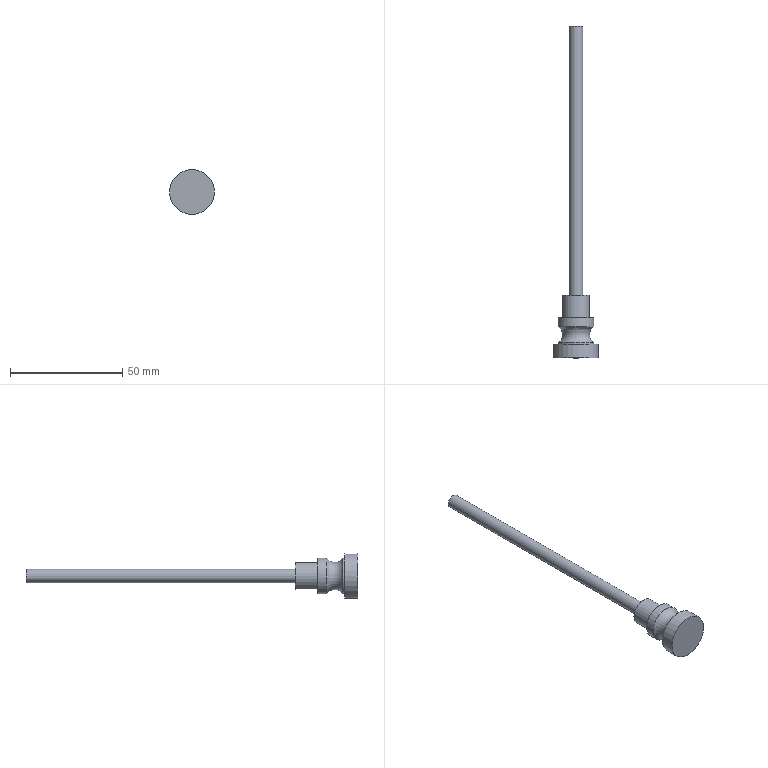Part | NX | features DATUM_CSYS 6, SKETCH 5, EXTRUDE 4, SWP104 1 | 1 solid | 11 faces | box 20 x 148 x 20 mm | volume 8375 mm3 | cylinder 5 | plane 5 | torus 1 | commonest cylinder face diameters 16 x2 6 x1 12 x1 20 x1
STEP:
#1=CARTESIAN_POINT('',(0.,0.721,8.));
#2=VERTEX_POINT('',#1);
#3=CARTESIAN_POINT('',(0.,0.721,0.));
#4=DIRECTION('',(0.,1.,0.));
#5=DIRECTION('',(0.,0.,1.));
#6=AXIS2_PLACEMENT_3D('',#3,#4,#5);
#7=CIRCLE('',#6,8.);
#8=EDGE_CURVE('',#2,#2,#7,.T.);
#9=ORIENTED_EDGE('',*,*,#8,.F.);
#10=EDGE_LOOP('',(#9));
#11=FACE_BOUND('',#10,.T.);
#12=CARTESIAN_POINT('',(8.,0.,0.));
#13=VERTEX_POINT('',#12);
#14=CARTESIAN_POINT('',(0.,0.,0.));
#15=DIRECTION('',(0.,1.,0.));
#16=DIRECTION('',(1.,0.,0.));
#17=AXIS2_PLACEMENT_3D('',#14,#15,#16);
#18=CIRCLE('',#17,8.);
#19=EDGE_CURVE('',#13,#13,#18,.T.);
#20=ORIENTED_EDGE('',*,*,#19,.T.);
#21=EDGE_LOOP('',(#20));
#22=FACE_BOUND('',#21,.T.);
#23=CARTESIAN_POINT('',(0.,12.,0.));
#24=DIRECTION('',(0.,-1.,0.));
#25=DIRECTION('',(0.,0.,-1.));
#26=AXIS2_PLACEMENT_3D('',#23,#24,#25);
#27=CYLINDRICAL_SURFACE('',#26,8.);
#28=ADVANCED_FACE('',(#11,#22),#27,.T.);
#29=CARTESIAN_POINT('',(10.,-6.,0.));
#30=VERTEX_POINT('',#29);
#31=CARTESIAN_POINT('',(0.,-6.,0.));
#32=DIRECTION('',(0.,-1.,0.));
#33=DIRECTION('',(1.,0.,0.));
#34=AXIS2_PLACEMENT_3D('',#31,#32,#33);
#35=CIRCLE('',#34,10.);
#36=EDGE_CURVE('',#30,#30,#35,.T.);
#37=ORIENTED_EDGE('',*,*,#36,.F.);
#38=EDGE_LOOP('',(#37));
#39=FACE_BOUND('',#38,.T.);
#40=CARTESIAN_POINT('',(10.,0.,0.));
#41=VERTEX_POINT('',#40);
#42=CARTESIAN_POINT('',(0.,0.,0.));
#43=DIRECTION('',(0.,-1.,0.));
#44=DIRECTION('',(1.,0.,0.));
#45=AXIS2_PLACEMENT_3D('',#42,#43,#44);
#46=CIRCLE('',#45,10.);
#47=EDGE_CURVE('',#41,#41,#46,.T.);
#48=ORIENTED_EDGE('',*,*,#47,.T.);
#49=EDGE_LOOP('',(#48));
#50=FACE_BOUND('',#49,.T.);
#51=CARTESIAN_POINT('',(0.,-6.,0.));
#52=DIRECTION('',(0.,1.,0.));
#53=DIRECTION('',(0.,0.,1.));
#54=AXIS2_PLACEMENT_3D('',#51,#52,#53);
#55=CYLINDRICAL_SURFACE('',#54,10.);
#56=ADVANCED_FACE('',(#39,#50),#55,.T.);
#57=ORIENTED_EDGE('',*,*,#36,.T.);
#58=EDGE_LOOP('',(#57));
#59=FACE_BOUND('',#58,.T.);
#60=CARTESIAN_POINT('',(0.,-6.,0.));
#61=DIRECTION('',(0.,-1.,0.));
#62=DIRECTION('',(0.,0.,-1.));
#63=AXIS2_PLACEMENT_3D('',#60,#61,#62);
#64=PLANE('',#63);
#65=ADVANCED_FACE('',(#59),#64,.T.);
#66=ORIENTED_EDGE('',*,*,#47,.F.);
#67=EDGE_LOOP('',(#66));
#68=FACE_BOUND('',#67,.T.);
#69=ORIENTED_EDGE('',*,*,#19,.F.);
#70=EDGE_LOOP('',(#69));
#71=FACE_BOUND('',#70,.T.);
#72=CARTESIAN_POINT('',(0.,0.,0.));
#73=DIRECTION('',(0.,-1.,0.));
#74=DIRECTION('',(0.,0.,-1.));
#75=AXIS2_PLACEMENT_3D('',#72,#73,#74);
#76=PLANE('',#75);
#77=ADVANCED_FACE('',(#68,#71),#76,.F.);
#78=CARTESIAN_POINT('',(0.,8.,-8.));
#79=VERTEX_POINT('',#78);
#80=CARTESIAN_POINT('',(0.,8.,0.));
#81=DIRECTION('',(0.,-1.,0.));
#82=DIRECTION('',(0.,0.,-1.));
#83=AXIS2_PLACEMENT_3D('',#80,#81,#82);
#84=CIRCLE('',#83,8.);
#85=EDGE_CURVE('',#79,#79,#84,.T.);
#86=ORIENTED_EDGE('',*,*,#85,.T.);
#87=EDGE_LOOP('',(#86));
#88=FACE_BOUND('',#87,.T.);
#89=ORIENTED_EDGE('',*,*,#8,.T.);
#90=EDGE_LOOP('',(#89));
#91=FACE_BOUND('',#90,.T.);
#92=CARTESIAN_POINT('',(0.,4.36,0.));
#93=DIRECTION('',(0.,-1.,0.));
#94=DIRECTION('',(0.,0.,-1.));
#95=AXIS2_PLACEMENT_3D('',#92,#93,#94);
#96=TOROIDAL_SURFACE('',#95,10.473,4.4);
#97=ADVANCED_FACE('',(#88,#91),#96,.F.);
#98=CARTESIAN_POINT('',(6.,12.,0.));
#99=VERTEX_POINT('',#98);
#100=CARTESIAN_POINT('',(0.,12.,0.));
#101=DIRECTION('',(0.,1.,0.));
#102=DIRECTION('',(1.,0.,0.));
#103=AXIS2_PLACEMENT_3D('',#100,#101,#102);
#104=CIRCLE('',#103,6.);
#105=EDGE_CURVE('',#99,#99,#104,.T.);
#106=ORIENTED_EDGE('',*,*,#105,.F.);
#107=EDGE_LOOP('',(#106));
#108=FACE_BOUND('',#107,.T.);
#109=CARTESIAN_POINT('',(8.,12.,0.));
#110=VERTEX_POINT('',#109);
#111=CARTESIAN_POINT('',(0.,12.,0.));
#112=DIRECTION('',(0.,1.,0.));
#113=DIRECTION('',(1.,0.,0.));
#114=AXIS2_PLACEMENT_3D('',#111,#112,#113);
#115=CIRCLE('',#114,8.);
#116=EDGE_CURVE('',#110,#110,#115,.T.);
#117=ORIENTED_EDGE('',*,*,#116,.T.);
#118=EDGE_LOOP('',(#117));
#119=FACE_BOUND('',#118,.T.);
#120=CARTESIAN_POINT('',(0.,12.,0.));
#121=DIRECTION('',(0.,1.,0.));
#122=DIRECTION('',(0.,0.,1.));
#123=AXIS2_PLACEMENT_3D('',#120,#121,#122);
#124=PLANE('',#123);
#125=ADVANCED_FACE('',(#108,#119),#124,.T.);
#126=ORIENTED_EDGE('',*,*,#85,.F.);
#127=EDGE_LOOP('',(#126));
#128=FACE_BOUND('',#127,.T.);
#129=ORIENTED_EDGE('',*,*,#116,.F.);
#130=EDGE_LOOP('',(#129));
#131=FACE_BOUND('',#130,.T.);
#132=CARTESIAN_POINT('',(0.,12.,0.));
#133=DIRECTION('',(0.,-1.,0.));
#134=DIRECTION('',(0.,0.,-1.));
#135=AXIS2_PLACEMENT_3D('',#132,#133,#134);
#136=CYLINDRICAL_SURFACE('',#135,8.);
#137=ADVANCED_FACE('',(#128,#131),#136,.T.);
#138=CARTESIAN_POINT('',(6.,22.,0.));
#139=VERTEX_POINT('',#138);
#140=CARTESIAN_POINT('',(0.,22.,0.));
#141=DIRECTION('',(0.,1.,0.));
#142=DIRECTION('',(1.,0.,0.));
#143=AXIS2_PLACEMENT_3D('',#140,#141,#142);
#144=CIRCLE('',#143,6.);
#145=EDGE_CURVE('',#139,#139,#144,.T.);
#146=ORIENTED_EDGE('',*,*,#145,.F.);
#147=EDGE_LOOP('',(#146));
#148=FACE_BOUND('',#147,.T.);
#149=ORIENTED_EDGE('',*,*,#105,.T.);
#150=EDGE_LOOP('',(#149));
#151=FACE_BOUND('',#150,.T.);
#152=CARTESIAN_POINT('',(0.,22.,0.));
#153=DIRECTION('',(0.,-1.,0.));
#154=DIRECTION('',(0.,0.,-1.));
#155=AXIS2_PLACEMENT_3D('',#152,#153,#154);
#156=CYLINDRICAL_SURFACE('',#155,6.);
#157=ADVANCED_FACE('',(#148,#151),#156,.T.);
#158=CARTESIAN_POINT('',(3.,22.,0.));
#159=VERTEX_POINT('',#158);
#160=CARTESIAN_POINT('',(0.,22.,0.));
#161=DIRECTION('',(0.,1.,0.));
#162=DIRECTION('',(1.,0.,0.));
#163=AXIS2_PLACEMENT_3D('',#160,#161,#162);
#164=CIRCLE('',#163,3.);
#165=EDGE_CURVE('',#159,#159,#164,.T.);
#166=ORIENTED_EDGE('',*,*,#165,.F.);
#167=EDGE_LOOP('',(#166));
#168=FACE_BOUND('',#167,.T.);
#169=ORIENTED_EDGE('',*,*,#145,.T.);
#170=EDGE_LOOP('',(#169));
#171=FACE_BOUND('',#170,.T.);
#172=CARTESIAN_POINT('',(0.,22.,0.));
#173=DIRECTION('',(0.,1.,0.));
#174=DIRECTION('',(0.,0.,1.));
#175=AXIS2_PLACEMENT_3D('',#172,#173,#174);
#176=PLANE('',#175);
#177=ADVANCED_FACE('',(#168,#171),#176,.T.);
#178=CARTESIAN_POINT('',(3.,142.,0.));
#179=VERTEX_POINT('',#178);
#180=CARTESIAN_POINT('',(0.,142.,0.));
#181=DIRECTION('',(0.,1.,0.));
#182=DIRECTION('',(1.,0.,0.));
#183=AXIS2_PLACEMENT_3D('',#180,#181,#182);
#184=CIRCLE('',#183,3.);
#185=EDGE_CURVE('',#179,#179,#184,.T.);
#186=ORIENTED_EDGE('',*,*,#185,.F.);
#187=EDGE_LOOP('',(#186));
#188=FACE_BOUND('',#187,.T.);
#189=ORIENTED_EDGE('',*,*,#165,.T.);
#190=EDGE_LOOP('',(#189));
#191=FACE_BOUND('',#190,.T.);
#192=CARTESIAN_POINT('',(0.,142.,0.));
#193=DIRECTION('',(0.,-1.,0.));
#194=DIRECTION('',(0.,0.,-1.));
#195=AXIS2_PLACEMENT_3D('',#192,#193,#194);
#196=CYLINDRICAL_SURFACE('',#195,3.);
#197=ADVANCED_FACE('',(#188,#191),#196,.T.);
#198=ORIENTED_EDGE('',*,*,#185,.T.);
#199=EDGE_LOOP('',(#198));
#200=FACE_BOUND('',#199,.T.);
#201=CARTESIAN_POINT('',(0.,142.,0.));
#202=DIRECTION('',(0.,1.,0.));
#203=DIRECTION('',(0.,0.,1.));
#204=AXIS2_PLACEMENT_3D('',#201,#202,#203);
#205=PLANE('',#204);
#206=ADVANCED_FACE('',(#200),#205,.T.);
#207=CLOSED_SHELL('',(#28,#56,#65,#77,#97,#125,#137,#157,#177,#197,#206));
#208=MANIFOLD_SOLID_BREP('',#207);
#209=(LENGTH_UNIT()NAMED_UNIT(*)SI_UNIT(.MILLI.,.METRE.));
#210=UNCERTAINTY_MEASURE_WITH_UNIT(LENGTH_MEASURE(0.00001),#209,'','');
#211=(NAMED_UNIT(*)PLANE_ANGLE_UNIT()SI_UNIT($,.RADIAN.));
#212=(NAMED_UNIT(*)SI_UNIT($,.STERADIAN.)SOLID_ANGLE_UNIT());
#213=(GEOMETRIC_REPRESENTATION_CONTEXT(3)GLOBAL_UNCERTAINTY_ASSIGNED_CONTEXT((#210))GLOBAL_UNIT_ASSIGNED_CONTEXT((#209,#211,#212))REPRESENTATION_CONTEXT('',''));
#214=ADVANCED_BREP_SHAPE_REPRESENTATION('',(#208),#213);